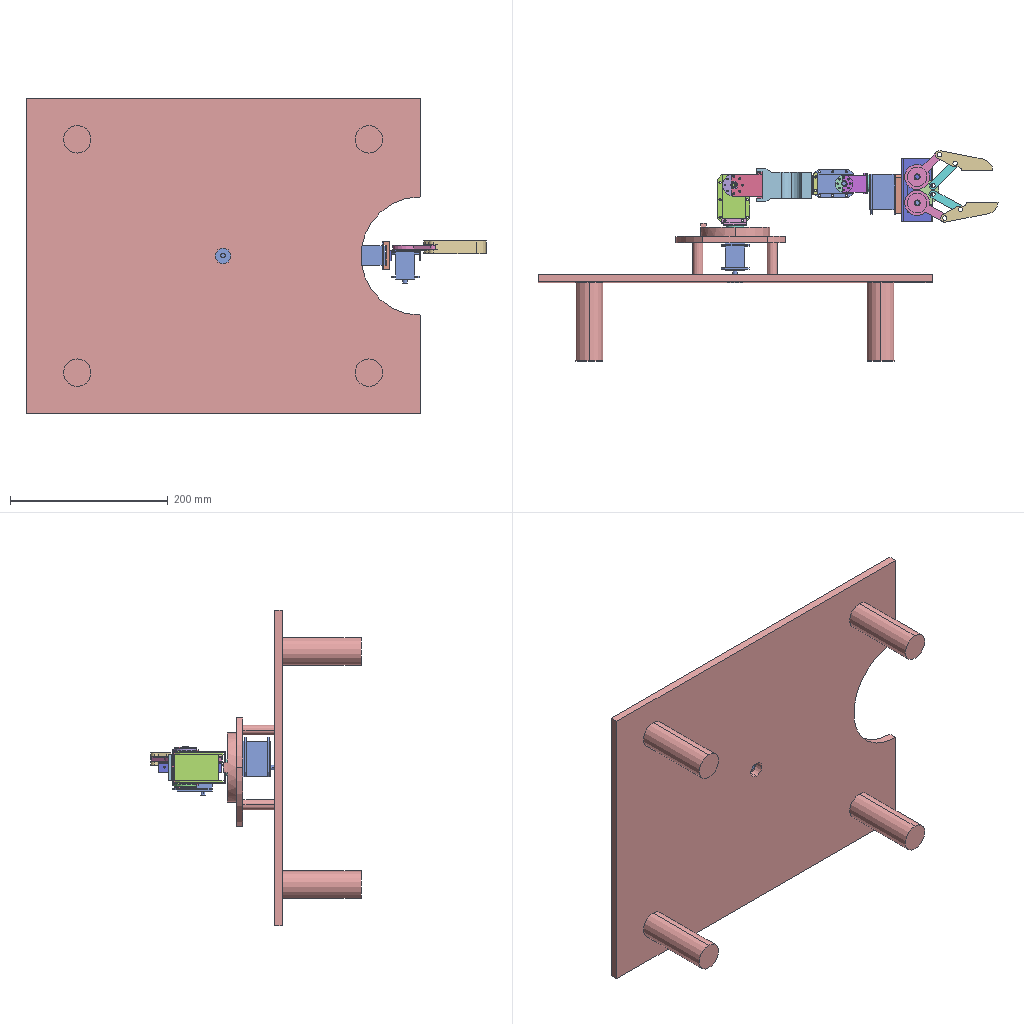Assembly | SolidWorks | 25 different items | 33 placed | box 584 x 267 x 400 mm
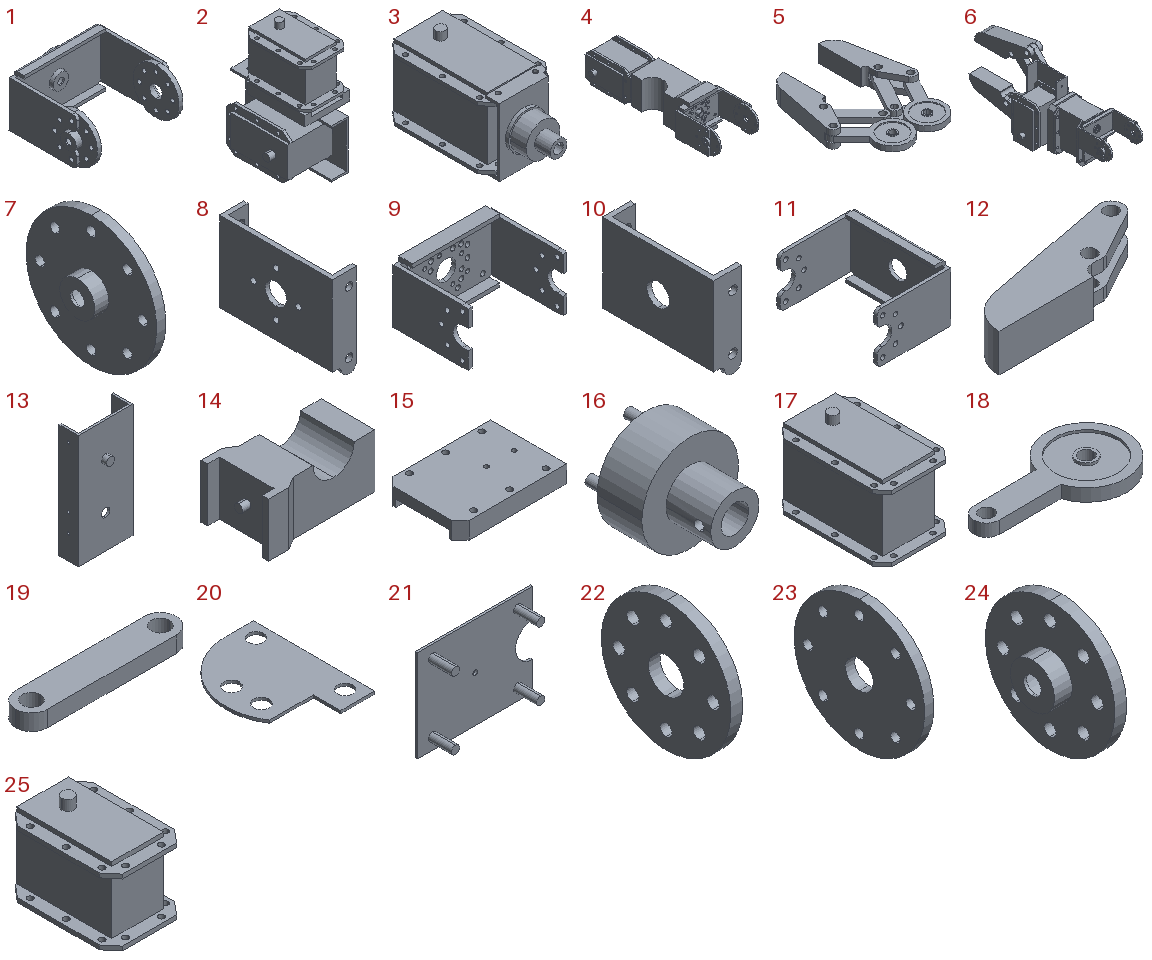Parts list (item | name | quantity | parent item | size | volume | features):
1 | (subassembly) | x1 | in 6 | 45.55 x 42.995 x 26 mm | 5773 mm3 | -
2 | (subassembly) | x1 | in 6 | 52.9 x 80 x 84.95 mm | 100199 mm3 | -
3 | (subassembly) | x1 | - | 40.2 x 84.8 x 47.35 mm | 75606 mm3 | -
4 | (subassembly) | x1 | - | 52 x 166 x 41.5 mm | 117123 mm3 | -
5 | (subassembly) | x1 | in 6 | 90.637 x 118.597 x 16 mm | 43192 mm3 | -
6 | (subassembly) | x1 | - | 56.883 x 206.393 x 90.637 mm | 149164 mm3 | -
7 | - | x1 | in 4 | 5 x 28 x 28 mm | 1183 mm3 | features BaseBody 1
8 | - | x1 | in 3 | 8.6 x 40 x 32 mm | 2244 mm3 | features BaseBody 1
9 | - | x1 | in 4 | 51 x 39 x 33 mm | 7566 mm3 | features BaseBody 1
10 | - | x1 | in 4 | 8.6 x 34.5 x 28 mm | 1746 mm3 | features BaseBody 1
11 | - | x1 | in 1 | 32.495 x 44 x 26 mm | 3696 mm3 | features BaseBody 1
12 | - | x2 | in 5 | 72.59 x 25.381 x 16 mm | 14653 mm3 | features BaseBody 1, ICE 1, MoveFace 1
13 | - | x1 | in 2 | 38.6 x 17 x 80 mm | 7545 mm3 | features BaseBody 1
14 | - | x1 | in 4 | 74.5 x 41.5 x 33 mm | 63883 mm3 | features BaseBody 1, ICE 1
15 | - | x1 | in 2 | 49.9 x 35.6 x 8 mm | 9414 mm3 | features BaseBody 1
16 | - | x1 | in 3 | 20 x 23.55 x 20 mm | 3677 mm3 | features BaseBody 1
17 | - | x1 | in 3 | 40.2 x 61.1 x 47.35 mm | 68973 mm3 | features BaseBody 1
18 | - | x2 | in 5 | 61 x 32 x 5 mm | 4287 mm3 | features BaseBody 1, ICE 1
19 | - | x2 | in 5 | 50 x 10 x 5 mm | 2138 mm3 | features BaseBody 1
20 | - | x1 | in 5 | 32.5 x 45 x 1 mm | 1036 mm3 | features BaseBody 1, ICE 1
21 | - | x1 | - | 500 x 175 x 400 mm | 2505450 mm3 | features ICE 2, BaseBody 1
22 | - | x1 | in 1 | 2 x 22 x 22 mm | 653.451 mm3 | features BaseBody 1
23 | - | x1 | in 4 | 2 x 28 x 28 mm | 1125 mm3 | features BaseBody 1
24 | - | x3 | in 1, 3 | 5 x 22 x 22 mm | 711.767 mm3 | features BaseBody 1
25 | - | x4 | in 2, 4 | 35.6 x 50.6 x 45.2 mm | 41620 mm3 | features BaseBody 1, ICE 1
Mates (type | each side: item.copy, entity, surface, feature):
In the top assembly
Concentric | 21.1 face cylinder Imported1 | 25.1 face cylinder Imported1
Parallel | 21.1 face plane Cut-Extrude1 | 25.1 face plane Imported1
Coincident | 21.1 face plane Imported1 | 25.1 face plane Imported1
Parallel | 21.1 face plane Cut-Extrude1 | 17.1 face plane Imported1
Concentric | 21.1 face cylinder Imported1 | 16.1 face cylinder Imported1
DistanceDim | 8.1 face plane Imported1 | 21.1 face plane Imported1
Width | 23.1 face plane Imported1 | 7.1 face plane Imported1 | 17.1 face plane Imported1 | 17.1 face plane Imported1
Concentric | 17.1 face cylinder Imported1 | 23.1 face cylinder Imported1
Parallel | 21.1 face plane Imported1 | 25.2 face plane Imported1
Concentric | 25.2 face cylinder Imported1 | 22.1 face cylinder Imported1
Width | 24.1 face plane Imported1 | 22.1 face plane Imported1 | 25.2 face plane Imported1 | 25.2 face plane Imported1
Parallel | 25.2 face plane Imported1 | 25.3 face plane Imported1
In subassembly 6
Concentric | 24.2 face cylinder Imported1 | 25.4 face cylinder Imported1
Coincident | 24.2 face plane Imported1 | 25.4 face plane Imported1
Parallel | 11.1 face plane Imported1 | 25.4 face plane Imported1
Concentric | 13.1 face cylinder Imported1 | 18.1 face cylinder Imported1
Concentric | 25.5 face cylinder Imported1 | 20.1 face cylinder Imported1
Coincident | 13.1 face plane Imported1 | 20.1 face plane Imported1
In subassembly 1
Concentric | 24.3 face cylinder Imported1 | 22.2 face cylinder Imported1
Concentric | 24.3 face cylinder Imported1 | 11.2 face cylinder Imported1 | 2 times
Coincident | 24.3 face plane Imported1 | 11.2 face plane Imported1
Coincident | 11.2 face plane Imported1 | 22.2 face plane Imported1
Concentric | 11.2 face cylinder Imported1 | 22.2 face cylinder Imported1
Concentric | 11.2 face cylinder Imported1 | 24.4 face cylinder Imported1
Coincident | 11.2 face plane Imported1 | 24.4 face plane Imported1
Parallel | 11.2 face plane Imported1 | 24.4 plane
In subassembly 5
Concentric | 20.2 face cylinder Imported1 | 18.2 face cylinder Imported1
Coincident | 20.2 face plane Imported1 | 18.2 face plane Imported1
Concentric | 20.2 face cylinder Imported1 | 19.1 face cylinder Imported1
Coincident | 20.2 face plane Imported1 | 19.1 face plane Imported1
Concentric | 19.1 face cylinder Imported1 | 12.1 face cylinder Imported1
Concentric | 18.2 face cylinder Imported1 | 12.1 face cylinder Boss-Extrude1
Width | 12.1 face plane Boss-Extrude1 | 12.1 face plane Imported1 | 19.1 face plane Imported1 | 19.1 face plane Imported1
Concentric | 20.2 face cylinder Imported1 | 19.2 face cylinder Imported1
Coincident | 20.2 face plane Imported1 | 19.2 face plane Imported1
Concentric | 20.2 face cylinder Imported1 | 18.3 face cylinder Imported1
Coincident | 20.2 face plane Imported1 | 18.3 face plane Imported1
Concentric | 18.3 face cylinder Imported1 | 12.2 face cylinder Boss-Extrude1
Concentric | 19.2 face cylinder Imported1 | 12.2 face cylinder Imported1
Width | 12.2 face plane Boss-Extrude1 | 12.2 face plane Imported1 | 19.2 face plane Imported1 | 19.2 face plane Imported1
GearDim | 18.2 face cylinder Imported1 | 18.3 face cylinder Imported1
PlanarAngleDim | 18.2 face plane Imported1 | 20.2 face plane Imported1
In subassembly 2
Coincident | 25.1 face plane Imported1 | 15.1 face plane Imported1
Concentric | 25.1 face cylinder Imported1 | 15.1 face cylinder Imported1 | 2 times
Coincident | 15.1 face plane Imported1 | 13.2 face plane Imported1
Concentric | 15.1 face cylinder Imported1 | 13.2 face cylinder Imported1 | 2 times
Coincident | 13.2 face plane Imported1 | 25.6 face plane Imported1 | 2 times
Concentric | 13.2 face cylinder Imported1 | 25.6 face cylinder Imported1
In subassembly 3
Concentric | 17.2 face cylinder Imported1 | 8.2 face cylinder Imported1 | 2 times
Coincident | 17.2 face plane Imported1 | 8.2 face plane Imported1
Concentric | 8.2 face cylinder Imported1 | 24.3 face cylinder Imported1 | 2 times
Coincident | 8.2 face plane Imported1 | 24.3 face plane Imported1
Concentric | 24.3 face cylinder Imported1 | 16.2 face cylinder Imported1 | 2 times
Coincident | 24.3 face plane Imported1 | 16.2 face plane Imported1
In subassembly 4
Concentric | 7.2 face cylinder Imported1 | 23.2 face cylinder Imported1 | 2 times
Coincident | 7.2 face plane Imported1 | 9.1 face plane Imported1
Concentric | 7.2 face cylinder Imported1 | 9.1 face cylinder Imported1 | 2 times
Coincident | 23.2 face plane Imported1 | 9.1 face plane Imported1
Coincident | 9.1 face plane Imported1 | 14.1 face plane Imported1
Concentric | 9.1 face cylinder Imported1 | 14.1 face cylinder Imported1
Parallel | 9.1 face plane Imported1 | 14.1 face plane Imported1
Concentric | 14.1 face cylinder Imported1 | 10.1 face cylinder Imported1
Coincident | 14.1 face plane Imported1 | 10.1 face plane Imported1
Coincident | 25.1 face plane Imported1 | 10.1 face plane Imported1
Concentric | 25.1 face cylinder Imported1 | 10.1 face cylinder Imported1 | 2 times